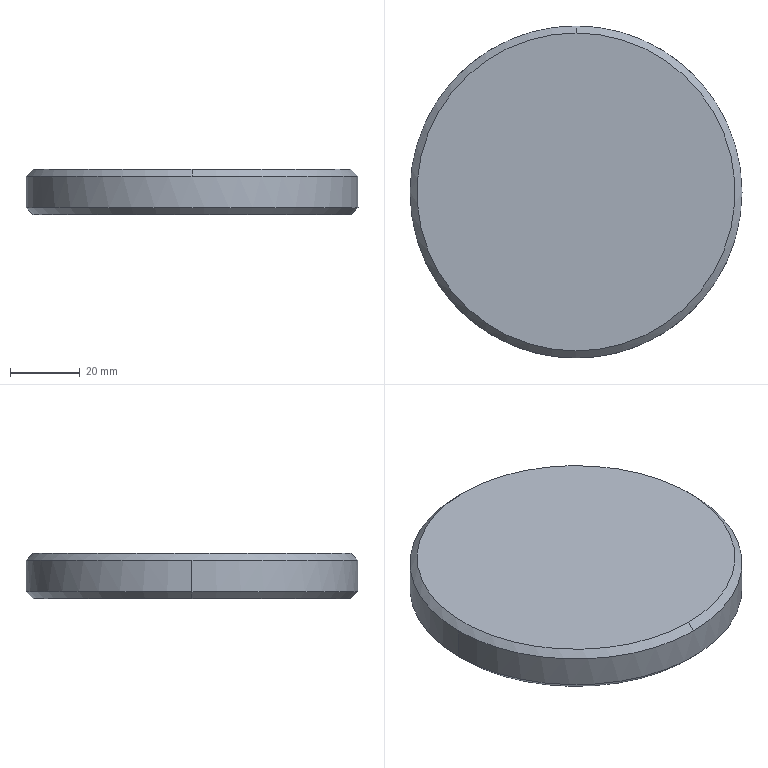Part | SolidWorks | features BaseBody 1 | 1 solid | 8 faces | box 95 x 95 x 13 mm | volume 90970 mm3 | cone 4 | cylinder 2 | plane 2 | commonest cylinder face diameters 95 x2
STEP:
#1=CARTESIAN_POINT('',(0.5253,44.067,13.));
#2=VERTEX_POINT('',#1);
#3=CARTESIAN_POINT('',(0.5253,-46.933,13.));
#4=VERTEX_POINT('',#3);
#5=CARTESIAN_POINT('',(0.5253,-1.433,13.));
#6=DIRECTION('',(0.,0.,-1.));
#7=DIRECTION('',(0.,1.,0.));
#8=AXIS2_PLACEMENT_3D('',#5,#6,#7);
#9=CIRCLE('',#8,45.5);
#10=EDGE_CURVE('',#2,#4,#9,.T.);
#11=ORIENTED_EDGE('',*,*,#10,.T.);
#12=CARTESIAN_POINT('',(0.5253,-48.933,11.));
#13=VERTEX_POINT('',#12);
#14=CARTESIAN_POINT('',(0.5253,-48.933,11.));
#15=DIRECTION('',(0.,-0.7071,-0.7071));
#16=VECTOR('',#15,1000.);
#17=LINE('',#14,#16);
#18=EDGE_CURVE('',#4,#13,#17,.T.);
#19=ORIENTED_EDGE('',*,*,#18,.T.);
#20=CARTESIAN_POINT('',(48.025,-1.433,11.));
#21=VERTEX_POINT('',#20);
#22=CARTESIAN_POINT('',(0.5253,-1.433,11.));
#23=DIRECTION('',(0.,0.,1.));
#24=DIRECTION('',(-1.,0.,0.));
#25=AXIS2_PLACEMENT_3D('',#22,#23,#24);
#26=CIRCLE('',#25,47.5);
#27=EDGE_CURVE('',#13,#21,#26,.T.);
#28=ORIENTED_EDGE('',*,*,#27,.T.);
#29=CARTESIAN_POINT('',(0.5253,46.067,11.));
#30=VERTEX_POINT('',#29);
#31=CARTESIAN_POINT('',(0.5253,-1.433,11.));
#32=DIRECTION('',(0.,0.,1.));
#33=DIRECTION('',(-1.,0.,0.));
#34=AXIS2_PLACEMENT_3D('',#31,#32,#33);
#35=CIRCLE('',#34,47.5);
#36=EDGE_CURVE('',#21,#30,#35,.T.);
#37=ORIENTED_EDGE('',*,*,#36,.T.);
#38=CARTESIAN_POINT('',(0.5253,46.067,11.));
#39=DIRECTION('',(0.,0.7071,-0.7071));
#40=VECTOR('',#39,1000.);
#41=LINE('',#38,#40);
#42=EDGE_CURVE('',#2,#30,#41,.T.);
#43=ORIENTED_EDGE('',*,*,#42,.F.);
#44=EDGE_LOOP('',(#11,#19,#28,#37,#43));
#45=FACE_OUTER_BOUND('',#44,.T.);
#46=CARTESIAN_POINT('',(0.5253,-1.433,11.));
#47=DIRECTION('',(0.,0.,-1.));
#48=DIRECTION('',(0.,1.,0.));
#49=AXIS2_PLACEMENT_3D('',#46,#47,#48);
#50=CONICAL_SURFACE('',#49,47.5,0.7854);
#51=ADVANCED_FACE('',(#45),#50,.T.);
#52=CARTESIAN_POINT('',(48.025,-1.433,2.));
#53=VERTEX_POINT('',#52);
#54=CARTESIAN_POINT('',(-46.975,-1.433,2.));
#55=VERTEX_POINT('',#54);
#56=CARTESIAN_POINT('',(0.5253,-1.433,2.));
#57=DIRECTION('',(0.,0.,1.));
#58=DIRECTION('',(1.,0.,0.));
#59=AXIS2_PLACEMENT_3D('',#56,#57,#58);
#60=CIRCLE('',#59,47.5);
#61=EDGE_CURVE('',#53,#55,#60,.T.);
#62=ORIENTED_EDGE('',*,*,#61,.T.);
#63=CARTESIAN_POINT('',(-46.975,-1.433,11.));
#64=VERTEX_POINT('',#63);
#65=CARTESIAN_POINT('',(-46.975,-1.433,0.));
#66=DIRECTION('',(0.,0.,1.));
#67=VECTOR('',#66,1000.);
#68=LINE('',#65,#67);
#69=EDGE_CURVE('',#55,#64,#68,.T.);
#70=ORIENTED_EDGE('',*,*,#69,.T.);
#71=CARTESIAN_POINT('',(0.5253,-1.433,11.));
#72=DIRECTION('',(0.,0.,1.));
#73=DIRECTION('',(-1.,0.,0.));
#74=AXIS2_PLACEMENT_3D('',#71,#72,#73);
#75=CIRCLE('',#74,47.5);
#76=EDGE_CURVE('',#30,#64,#75,.T.);
#77=ORIENTED_EDGE('',*,*,#76,.F.);
#78=ORIENTED_EDGE('',*,*,#36,.F.);
#79=CARTESIAN_POINT('',(48.025,-1.433,0.));
#80=DIRECTION('',(0.,0.,1.));
#81=VECTOR('',#80,1000.);
#82=LINE('',#79,#81);
#83=EDGE_CURVE('',#53,#21,#82,.T.);
#84=ORIENTED_EDGE('',*,*,#83,.F.);
#85=EDGE_LOOP('',(#62,#70,#77,#78,#84));
#86=FACE_OUTER_BOUND('',#85,.T.);
#87=CARTESIAN_POINT('',(0.5253,-1.433,0.));
#88=DIRECTION('',(0.,0.,1.));
#89=DIRECTION('',(1.,0.,0.));
#90=AXIS2_PLACEMENT_3D('',#87,#88,#89);
#91=CYLINDRICAL_SURFACE('',#90,47.5);
#92=ADVANCED_FACE('',(#86),#91,.T.);
#93=CARTESIAN_POINT('',(46.025,-1.433,0.));
#94=VERTEX_POINT('',#93);
#95=CARTESIAN_POINT('',(-44.975,-1.433,0.));
#96=VERTEX_POINT('',#95);
#97=CARTESIAN_POINT('',(0.5253,-1.433,0.));
#98=DIRECTION('',(0.,0.,1.));
#99=DIRECTION('',(1.,0.,0.));
#100=AXIS2_PLACEMENT_3D('',#97,#98,#99);
#101=CIRCLE('',#100,45.5);
#102=EDGE_CURVE('',#94,#96,#101,.T.);
#103=ORIENTED_EDGE('',*,*,#102,.T.);
#104=CARTESIAN_POINT('',(-46.975,-1.433,2.));
#105=DIRECTION('',(-0.7071,0.,0.7071));
#106=VECTOR('',#105,1000.);
#107=LINE('',#104,#106);
#108=EDGE_CURVE('',#96,#55,#107,.T.);
#109=ORIENTED_EDGE('',*,*,#108,.T.);
#110=ORIENTED_EDGE('',*,*,#61,.F.);
#111=CARTESIAN_POINT('',(48.025,-1.433,2.));
#112=DIRECTION('',(0.7071,0.,0.7071));
#113=VECTOR('',#112,1000.);
#114=LINE('',#111,#113);
#115=EDGE_CURVE('',#94,#53,#114,.T.);
#116=ORIENTED_EDGE('',*,*,#115,.F.);
#117=EDGE_LOOP('',(#103,#109,#110,#116));
#118=FACE_OUTER_BOUND('',#117,.T.);
#119=CARTESIAN_POINT('',(0.5253,-1.433,2.));
#120=DIRECTION('',(0.,0.,1.));
#121=DIRECTION('',(1.,0.,0.));
#122=AXIS2_PLACEMENT_3D('',#119,#120,#121);
#123=CONICAL_SURFACE('',#122,47.5,0.7854);
#124=ADVANCED_FACE('',(#118),#123,.T.);
#125=ORIENTED_EDGE('',*,*,#10,.F.);
#126=CARTESIAN_POINT('',(0.5253,-1.433,13.));
#127=DIRECTION('',(0.,0.,-1.));
#128=DIRECTION('',(0.,1.,0.));
#129=AXIS2_PLACEMENT_3D('',#126,#127,#128);
#130=CIRCLE('',#129,45.5);
#131=EDGE_CURVE('',#4,#2,#130,.T.);
#132=ORIENTED_EDGE('',*,*,#131,.F.);
#133=EDGE_LOOP('',(#125,#132));
#134=FACE_OUTER_BOUND('',#133,.T.);
#135=CARTESIAN_POINT('',(0.5253,-1.433,13.));
#136=DIRECTION('',(0.,0.,-1.));
#137=DIRECTION('',(-1.,0.,0.));
#138=AXIS2_PLACEMENT_3D('',#135,#136,#137);
#139=PLANE('',#138);
#140=ADVANCED_FACE('',(#134),#139,.F.);
#141=ORIENTED_EDGE('',*,*,#18,.F.);
#142=ORIENTED_EDGE('',*,*,#131,.T.);
#143=ORIENTED_EDGE('',*,*,#42,.T.);
#144=ORIENTED_EDGE('',*,*,#76,.T.);
#145=CARTESIAN_POINT('',(0.5253,-1.433,11.));
#146=DIRECTION('',(0.,0.,1.));
#147=DIRECTION('',(-1.,0.,0.));
#148=AXIS2_PLACEMENT_3D('',#145,#146,#147);
#149=CIRCLE('',#148,47.5);
#150=EDGE_CURVE('',#64,#13,#149,.T.);
#151=ORIENTED_EDGE('',*,*,#150,.T.);
#152=EDGE_LOOP('',(#141,#142,#143,#144,#151));
#153=FACE_OUTER_BOUND('',#152,.T.);
#154=CARTESIAN_POINT('',(0.5253,-1.433,11.));
#155=DIRECTION('',(0.,0.,-1.));
#156=DIRECTION('',(0.,1.,0.));
#157=AXIS2_PLACEMENT_3D('',#154,#155,#156);
#158=CONICAL_SURFACE('',#157,47.5,0.7854);
#159=ADVANCED_FACE('',(#153),#158,.T.);
#160=ORIENTED_EDGE('',*,*,#69,.F.);
#161=CARTESIAN_POINT('',(0.5253,-1.433,2.));
#162=DIRECTION('',(0.,0.,1.));
#163=DIRECTION('',(1.,0.,0.));
#164=AXIS2_PLACEMENT_3D('',#161,#162,#163);
#165=CIRCLE('',#164,47.5);
#166=EDGE_CURVE('',#55,#53,#165,.T.);
#167=ORIENTED_EDGE('',*,*,#166,.T.);
#168=ORIENTED_EDGE('',*,*,#83,.T.);
#169=ORIENTED_EDGE('',*,*,#27,.F.);
#170=ORIENTED_EDGE('',*,*,#150,.F.);
#171=EDGE_LOOP('',(#160,#167,#168,#169,#170));
#172=FACE_OUTER_BOUND('',#171,.T.);
#173=CARTESIAN_POINT('',(0.5253,-1.433,0.));
#174=DIRECTION('',(0.,0.,1.));
#175=DIRECTION('',(1.,0.,0.));
#176=AXIS2_PLACEMENT_3D('',#173,#174,#175);
#177=CYLINDRICAL_SURFACE('',#176,47.5);
#178=ADVANCED_FACE('',(#172),#177,.T.);
#179=ORIENTED_EDGE('',*,*,#108,.F.);
#180=CARTESIAN_POINT('',(0.5253,-1.433,0.));
#181=DIRECTION('',(0.,0.,1.));
#182=DIRECTION('',(1.,0.,0.));
#183=AXIS2_PLACEMENT_3D('',#180,#181,#182);
#184=CIRCLE('',#183,45.5);
#185=EDGE_CURVE('',#96,#94,#184,.T.);
#186=ORIENTED_EDGE('',*,*,#185,.T.);
#187=ORIENTED_EDGE('',*,*,#115,.T.);
#188=ORIENTED_EDGE('',*,*,#166,.F.);
#189=EDGE_LOOP('',(#179,#186,#187,#188));
#190=FACE_OUTER_BOUND('',#189,.T.);
#191=CARTESIAN_POINT('',(0.5253,-1.433,2.));
#192=DIRECTION('',(0.,0.,1.));
#193=DIRECTION('',(1.,0.,0.));
#194=AXIS2_PLACEMENT_3D('',#191,#192,#193);
#195=CONICAL_SURFACE('',#194,47.5,0.7854);
#196=ADVANCED_FACE('',(#190),#195,.T.);
#197=ORIENTED_EDGE('',*,*,#102,.F.);
#198=ORIENTED_EDGE('',*,*,#185,.F.);
#199=EDGE_LOOP('',(#197,#198));
#200=FACE_OUTER_BOUND('',#199,.T.);
#201=CARTESIAN_POINT('',(0.5253,-1.433,0.));
#202=DIRECTION('',(0.,0.,-1.));
#203=DIRECTION('',(-1.,0.,0.));
#204=AXIS2_PLACEMENT_3D('',#201,#202,#203);
#205=PLANE('',#204);
#206=ADVANCED_FACE('',(#200),#205,.T.);
#207=CLOSED_SHELL('',(#51,#92,#124,#140,#159,#178,#196,#206));
#208=MANIFOLD_SOLID_BREP('',#207);
#209=CARTESIAN_POINT('',(0.,0.,0.));
#210=DIRECTION('',(0.,0.,1.));
#211=DIRECTION('',(1.,0.,0.));
#212=AXIS2_PLACEMENT_3D('',#209,#210,#211);
#213=(LENGTH_UNIT()NAMED_UNIT(*)SI_UNIT(.MILLI.,.METRE.));
#214=UNCERTAINTY_MEASURE_WITH_UNIT(LENGTH_MEASURE(0.00001),#213,'','');
#215=(NAMED_UNIT(*)PLANE_ANGLE_UNIT()SI_UNIT($,.RADIAN.));
#216=(NAMED_UNIT(*)SI_UNIT($,.STERADIAN.)SOLID_ANGLE_UNIT());
#217=(GEOMETRIC_REPRESENTATION_CONTEXT(3)GLOBAL_UNCERTAINTY_ASSIGNED_CONTEXT((#214))GLOBAL_UNIT_ASSIGNED_CONTEXT((#213,#215,#216))REPRESENTATION_CONTEXT('',''));
#218=ADVANCED_BREP_SHAPE_REPRESENTATION('',(#208,#212),#217);